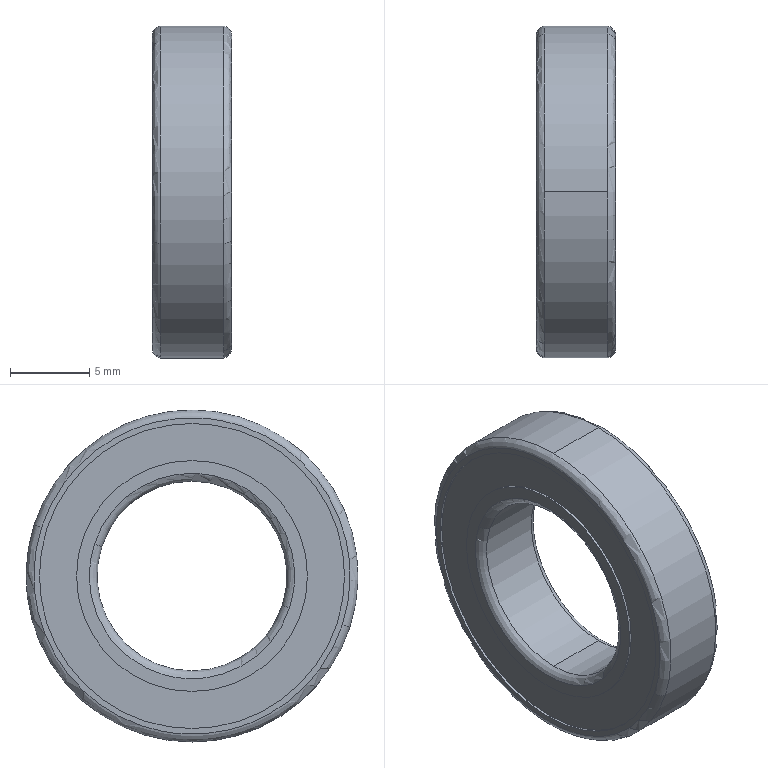Part | SolidWorks | features BaseBody 16 | 16 solids | 72 faces | box 5 x 21 x 21 mm | volume 741.464 mm3 | cylinder 24 | sphere 24 | torus 14 | plane 10 | commonest cylinder face diameters 14.6 x8 19.3 x8 18.4 x4 12 x2 21 x2